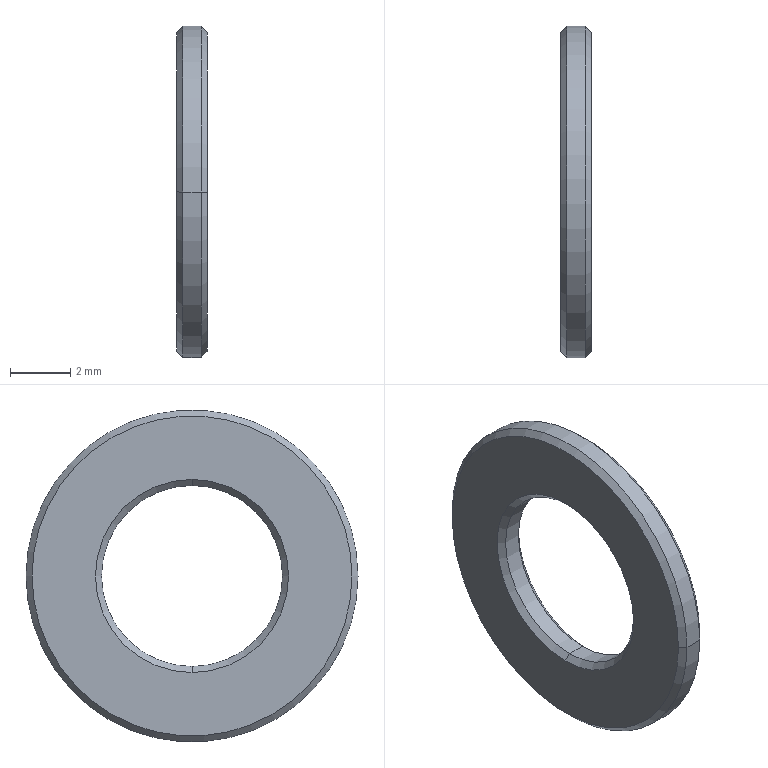Part | STEP file | FWSSS-D11-V6-T1 | 1 solid | 14 faces | box 1 x 11 x 11 mm | volume 64.623 mm3 | cone 8 | cylinder 4 | plane 2 | commonest cylinder face diameters 6 x2 11 x2
STEP:
#1=CARTESIAN_POINT('',(0.,0.,0.));
#2=DIRECTION('',(0.,0.,1.));
#3=DIRECTION('',(1.,0.,0.));
#4=AXIS2_PLACEMENT_3D('',#1,#2,#3);
#5=CARTESIAN_POINT('',(0.2,0.,3.));
#6=VERTEX_POINT('',#5);
#7=CARTESIAN_POINT('',(0.,0.,3.2));
#8=VERTEX_POINT('',#7);
#9=CARTESIAN_POINT('',(0.2,0.,3.));
#10=DIRECTION('',(-0.7071,0.,0.7071));
#11=VECTOR('',#10,1.);
#12=LINE('',#9,#11);
#13=CARTESIAN_POINT('',(0.2,0.,0.));
#14=DIRECTION('',(-1.,0.,0.));
#15=DIRECTION('',(0.,0.,1.));
#16=AXIS2_PLACEMENT_3D('',#13,#14,#15);
#17=CONICAL_SURFACE('',#16,3.,0.7854);
#18=CARTESIAN_POINT('',(6.283,0.));
#19=DIRECTION('',(0.,1.));
#20=VECTOR('',#19,1.);
#21=LINE('',#18,#20);
#22=(GEOMETRIC_REPRESENTATION_CONTEXT(2)PARAMETRIC_REPRESENTATION_CONTEXT()REPRESENTATION_CONTEXT('',''));
#23=DEFINITIONAL_REPRESENTATION('',(#21),#22);
#24=PCURVE('',#17,#23);
#25=CARTESIAN_POINT('',(0.2,0.,0.));
#26=DIRECTION('',(-1.,0.,0.));
#27=DIRECTION('',(0.,0.,1.));
#28=AXIS2_PLACEMENT_3D('',#25,#26,#27);
#29=CONICAL_SURFACE('',#28,3.,0.7854);
#30=CARTESIAN_POINT('',(0.,0.));
#31=DIRECTION('',(0.,1.));
#32=VECTOR('',#31,1.);
#33=LINE('',#30,#32);
#34=(GEOMETRIC_REPRESENTATION_CONTEXT(2)PARAMETRIC_REPRESENTATION_CONTEXT()REPRESENTATION_CONTEXT('',''));
#35=DEFINITIONAL_REPRESENTATION('',(#33),#34);
#36=PCURVE('',#29,#35);
#37=SURFACE_CURVE('',#12,(#24,#36),.PCURVE_S1.);
#38=EDGE_CURVE('',#6,#8,#37,.T.);
#39=ORIENTED_EDGE('',*,*,#38,.T.);
#40=CARTESIAN_POINT('',(0.,0.,-3.2));
#41=VERTEX_POINT('',#40);
#42=CARTESIAN_POINT('',(0.,0.,0.));
#43=DIRECTION('',(1.,0.,0.));
#44=DIRECTION('',(0.,1.,0.));
#45=AXIS2_PLACEMENT_3D('',#42,#43,#44);
#46=CIRCLE('',#45,3.2);
#47=CARTESIAN_POINT('',(7.854,0.2));
#48=DIRECTION('',(-1.,0.));
#49=VECTOR('',#48,1.);
#50=LINE('',#47,#49);
#51=(GEOMETRIC_REPRESENTATION_CONTEXT(2)PARAMETRIC_REPRESENTATION_CONTEXT()REPRESENTATION_CONTEXT('',''));
#52=DEFINITIONAL_REPRESENTATION('',(#50),#51);
#53=PCURVE('',#17,#52);
#54=CARTESIAN_POINT('',(0.,5.5,0.));
#55=DIRECTION('',(1.,0.,0.));
#56=DIRECTION('',(0.,1.,0.));
#57=AXIS2_PLACEMENT_3D('',#54,#55,#56);
#58=PLANE('',#57);
#59=CARTESIAN_POINT('',(-5.5,0.));
#60=DIRECTION('',(1.,0.));
#61=AXIS2_PLACEMENT_2D('',#59,#60);
#62=CIRCLE('',#61,3.2);
#63=(GEOMETRIC_REPRESENTATION_CONTEXT(2)PARAMETRIC_REPRESENTATION_CONTEXT()REPRESENTATION_CONTEXT('',''));
#64=DEFINITIONAL_REPRESENTATION('',(#62),#63);
#65=PCURVE('',#58,#64);
#66=SURFACE_CURVE('',#46,(#53,#65),.PCURVE_S1.);
#67=EDGE_CURVE('',#8,#41,#66,.T.);
#68=ORIENTED_EDGE('',*,*,#67,.T.);
#69=CARTESIAN_POINT('',(0.2,0.,-3.));
#70=VERTEX_POINT('',#69);
#71=CARTESIAN_POINT('',(0.2,0.,-3.));
#72=DIRECTION('',(-0.7071,0.,-0.7071));
#73=VECTOR('',#72,1.);
#74=LINE('',#71,#73);
#75=CARTESIAN_POINT('',(3.142,0.));
#76=DIRECTION('',(0.,1.));
#77=VECTOR('',#76,1.);
#78=LINE('',#75,#77);
#79=(GEOMETRIC_REPRESENTATION_CONTEXT(2)PARAMETRIC_REPRESENTATION_CONTEXT()REPRESENTATION_CONTEXT('',''));
#80=DEFINITIONAL_REPRESENTATION('',(#78),#79);
#81=PCURVE('',#17,#80);
#82=CARTESIAN_POINT('',(3.142,0.));
#83=DIRECTION('',(0.,1.));
#84=VECTOR('',#83,1.);
#85=LINE('',#82,#84);
#86=(GEOMETRIC_REPRESENTATION_CONTEXT(2)PARAMETRIC_REPRESENTATION_CONTEXT()REPRESENTATION_CONTEXT('',''));
#87=DEFINITIONAL_REPRESENTATION('',(#85),#86);
#88=PCURVE('',#29,#87);
#89=SURFACE_CURVE('',#74,(#81,#88),.PCURVE_S1.);
#90=EDGE_CURVE('',#70,#41,#89,.T.);
#91=ORIENTED_EDGE('',*,*,#90,.F.);
#92=CARTESIAN_POINT('',(0.2,0.,0.));
#93=DIRECTION('',(-1.,0.,0.));
#94=DIRECTION('',(0.,0.,-1.));
#95=AXIS2_PLACEMENT_3D('',#92,#93,#94);
#96=CIRCLE('',#95,3.);
#97=CARTESIAN_POINT('',(3.142,0.));
#98=DIRECTION('',(1.,0.));
#99=VECTOR('',#98,1.);
#100=LINE('',#97,#99);
#101=(GEOMETRIC_REPRESENTATION_CONTEXT(2)PARAMETRIC_REPRESENTATION_CONTEXT()REPRESENTATION_CONTEXT('',''));
#102=DEFINITIONAL_REPRESENTATION('',(#100),#101);
#103=PCURVE('',#17,#102);
#104=CARTESIAN_POINT('',(0.,0.,0.));
#105=DIRECTION('',(1.,0.,0.));
#106=DIRECTION('',(0.,0.,-1.));
#107=AXIS2_PLACEMENT_3D('',#104,#105,#106);
#108=CYLINDRICAL_SURFACE('',#107,3.);
#109=CARTESIAN_POINT('',(6.283,0.2));
#110=DIRECTION('',(-1.,0.));
#111=VECTOR('',#110,1.);
#112=LINE('',#109,#111);
#113=(GEOMETRIC_REPRESENTATION_CONTEXT(2)PARAMETRIC_REPRESENTATION_CONTEXT()REPRESENTATION_CONTEXT('',''));
#114=DEFINITIONAL_REPRESENTATION('',(#112),#113);
#115=PCURVE('',#108,#114);
#116=SURFACE_CURVE('',#96,(#103,#115),.PCURVE_S1.);
#117=EDGE_CURVE('',#70,#6,#116,.T.);
#118=ORIENTED_EDGE('',*,*,#117,.T.);
#119=EDGE_LOOP('',(#39,#68,#91,#118));
#120=FACE_BOUND('',#119,.F.);
#121=ADVANCED_FACE('',(#120),#17,.F.);
#122=CARTESIAN_POINT('',(0.8,0.,-3.));
#123=VERTEX_POINT('',#122);
#124=CARTESIAN_POINT('',(1.,0.,-3.2));
#125=VERTEX_POINT('',#124);
#126=CARTESIAN_POINT('',(0.8,0.,-3.));
#127=DIRECTION('',(0.7071,0.,-0.7071));
#128=VECTOR('',#127,1.);
#129=LINE('',#126,#128);
#130=CARTESIAN_POINT('',(0.8,0.,0.));
#131=DIRECTION('',(1.,0.,0.));
#132=DIRECTION('',(0.,0.,-1.));
#133=AXIS2_PLACEMENT_3D('',#130,#131,#132);
#134=CONICAL_SURFACE('',#133,3.,0.7854);
#135=CARTESIAN_POINT('',(6.283,0.));
#136=DIRECTION('',(0.,1.));
#137=VECTOR('',#136,1.);
#138=LINE('',#135,#137);
#139=(GEOMETRIC_REPRESENTATION_CONTEXT(2)PARAMETRIC_REPRESENTATION_CONTEXT()REPRESENTATION_CONTEXT('',''));
#140=DEFINITIONAL_REPRESENTATION('',(#138),#139);
#141=PCURVE('',#134,#140);
#142=CARTESIAN_POINT('',(0.8,0.,0.));
#143=DIRECTION('',(1.,0.,0.));
#144=DIRECTION('',(0.,0.,-1.));
#145=AXIS2_PLACEMENT_3D('',#142,#143,#144);
#146=CONICAL_SURFACE('',#145,3.,0.7854);
#147=CARTESIAN_POINT('',(0.,0.));
#148=DIRECTION('',(0.,1.));
#149=VECTOR('',#148,1.);
#150=LINE('',#147,#149);
#151=(GEOMETRIC_REPRESENTATION_CONTEXT(2)PARAMETRIC_REPRESENTATION_CONTEXT()REPRESENTATION_CONTEXT('',''));
#152=DEFINITIONAL_REPRESENTATION('',(#150),#151);
#153=PCURVE('',#146,#152);
#154=SURFACE_CURVE('',#129,(#141,#153),.PCURVE_S1.);
#155=EDGE_CURVE('',#123,#125,#154,.T.);
#156=ORIENTED_EDGE('',*,*,#155,.T.);
#157=CARTESIAN_POINT('',(1.,0.,3.2));
#158=VERTEX_POINT('',#157);
#159=CARTESIAN_POINT('',(1.,0.,0.));
#160=DIRECTION('',(-1.,0.,0.));
#161=DIRECTION('',(0.,-1.,0.));
#162=AXIS2_PLACEMENT_3D('',#159,#160,#161);
#163=CIRCLE('',#162,3.2);
#164=CARTESIAN_POINT('',(10.996,0.2));
#165=DIRECTION('',(-1.,0.));
#166=VECTOR('',#165,1.);
#167=LINE('',#164,#166);
#168=(GEOMETRIC_REPRESENTATION_CONTEXT(2)PARAMETRIC_REPRESENTATION_CONTEXT()REPRESENTATION_CONTEXT('',''));
#169=DEFINITIONAL_REPRESENTATION('',(#167),#168);
#170=PCURVE('',#134,#169);
#171=CARTESIAN_POINT('',(1.,5.5,0.));
#172=DIRECTION('',(-1.,0.,0.));
#173=DIRECTION('',(0.,-1.,0.));
#174=AXIS2_PLACEMENT_3D('',#171,#172,#173);
#175=PLANE('',#174);
#176=CARTESIAN_POINT('',(5.5,0.));
#177=DIRECTION('',(1.,0.));
#178=AXIS2_PLACEMENT_2D('',#176,#177);
#179=CIRCLE('',#178,3.2);
#180=(GEOMETRIC_REPRESENTATION_CONTEXT(2)PARAMETRIC_REPRESENTATION_CONTEXT()REPRESENTATION_CONTEXT('',''));
#181=DEFINITIONAL_REPRESENTATION('',(#179),#180);
#182=PCURVE('',#175,#181);
#183=SURFACE_CURVE('',#163,(#170,#182),.PCURVE_S1.);
#184=EDGE_CURVE('',#125,#158,#183,.T.);
#185=ORIENTED_EDGE('',*,*,#184,.T.);
#186=CARTESIAN_POINT('',(0.8,0.,3.));
#187=VERTEX_POINT('',#186);
#188=CARTESIAN_POINT('',(0.8,0.,3.));
#189=DIRECTION('',(0.7071,0.,0.7071));
#190=VECTOR('',#189,1.);
#191=LINE('',#188,#190);
#192=CARTESIAN_POINT('',(3.142,0.));
#193=DIRECTION('',(0.,1.));
#194=VECTOR('',#193,1.);
#195=LINE('',#192,#194);
#196=(GEOMETRIC_REPRESENTATION_CONTEXT(2)PARAMETRIC_REPRESENTATION_CONTEXT()REPRESENTATION_CONTEXT('',''));
#197=DEFINITIONAL_REPRESENTATION('',(#195),#196);
#198=PCURVE('',#134,#197);
#199=CARTESIAN_POINT('',(3.142,0.));
#200=DIRECTION('',(0.,1.));
#201=VECTOR('',#200,1.);
#202=LINE('',#199,#201);
#203=(GEOMETRIC_REPRESENTATION_CONTEXT(2)PARAMETRIC_REPRESENTATION_CONTEXT()REPRESENTATION_CONTEXT('',''));
#204=DEFINITIONAL_REPRESENTATION('',(#202),#203);
#205=PCURVE('',#146,#204);
#206=SURFACE_CURVE('',#191,(#198,#205),.PCURVE_S1.);
#207=EDGE_CURVE('',#187,#158,#206,.T.);
#208=ORIENTED_EDGE('',*,*,#207,.F.);
#209=CARTESIAN_POINT('',(0.8,0.,0.));
#210=DIRECTION('',(1.,0.,0.));
#211=DIRECTION('',(0.,0.,1.));
#212=AXIS2_PLACEMENT_3D('',#209,#210,#211);
#213=CIRCLE('',#212,3.);
#214=CARTESIAN_POINT('',(3.142,0.));
#215=DIRECTION('',(1.,0.));
#216=VECTOR('',#215,1.);
#217=LINE('',#214,#216);
#218=(GEOMETRIC_REPRESENTATION_CONTEXT(2)PARAMETRIC_REPRESENTATION_CONTEXT()REPRESENTATION_CONTEXT('',''));
#219=DEFINITIONAL_REPRESENTATION('',(#217),#218);
#220=PCURVE('',#134,#219);
#221=CARTESIAN_POINT('',(3.142,0.8));
#222=DIRECTION('',(1.,0.));
#223=VECTOR('',#222,1.);
#224=LINE('',#221,#223);
#225=(GEOMETRIC_REPRESENTATION_CONTEXT(2)PARAMETRIC_REPRESENTATION_CONTEXT()REPRESENTATION_CONTEXT('',''));
#226=DEFINITIONAL_REPRESENTATION('',(#224),#225);
#227=PCURVE('',#108,#226);
#228=SURFACE_CURVE('',#213,(#220,#227),.PCURVE_S1.);
#229=EDGE_CURVE('',#187,#123,#228,.T.);
#230=ORIENTED_EDGE('',*,*,#229,.T.);
#231=EDGE_LOOP('',(#156,#185,#208,#230));
#232=FACE_BOUND('',#231,.F.);
#233=ADVANCED_FACE('',(#232),#134,.F.);
#234=CARTESIAN_POINT('',(1.,5.3,0.));
#235=VERTEX_POINT('',#234);
#236=CARTESIAN_POINT('',(1.,-5.3,0.));
#237=VERTEX_POINT('',#236);
#238=CARTESIAN_POINT('',(1.,0.,0.));
#239=DIRECTION('',(1.,0.,0.));
#240=DIRECTION('',(0.,-1.,0.));
#241=AXIS2_PLACEMENT_3D('',#238,#239,#240);
#242=CIRCLE('',#241,5.3);
#243=CARTESIAN_POINT('',(0.8,0.,0.));
#244=DIRECTION('',(-1.,0.,0.));
#245=DIRECTION('',(0.,-1.,0.));
#246=AXIS2_PLACEMENT_3D('',#243,#244,#245);
#247=CONICAL_SURFACE('',#246,5.5,0.7854);
#248=CARTESIAN_POINT('',(6.283,-0.2));
#249=DIRECTION('',(-1.,0.));
#250=VECTOR('',#249,1.);
#251=LINE('',#248,#250);
#252=(GEOMETRIC_REPRESENTATION_CONTEXT(2)PARAMETRIC_REPRESENTATION_CONTEXT()REPRESENTATION_CONTEXT('',''));
#253=DEFINITIONAL_REPRESENTATION('',(#251),#252);
#254=PCURVE('',#247,#253);
#255=CARTESIAN_POINT('',(10.8,0.));
#256=CARTESIAN_POINT('',(10.8,-9.18));
#257=CARTESIAN_POINT('',(2.85,-4.59));
#258=CARTESIAN_POINT('',(-5.1,0.));
#259=CARTESIAN_POINT('',(2.85,4.59));
#260=CARTESIAN_POINT('',(10.8,9.18));
#261=CARTESIAN_POINT('',(10.8,0.));
#262=(BOUNDED_CURVE()B_SPLINE_CURVE(2,(#255,#256,#257,#258,#259,#260,#261),.UNSPECIFIED.,.T.,.F.)B_SPLINE_CURVE_WITH_KNOTS((1,2,2,2,2,1),(-2.094,0.,2.094,4.189,6.283,8.378),.UNSPECIFIED.)CURVE()GEOMETRIC_REPRESENTATION_ITEM()RATIONAL_B_SPLINE_CURVE((1.,0.5,1.,0.5,1.,0.5,1.))REPRESENTATION_ITEM(''));
#263=(GEOMETRIC_REPRESENTATION_CONTEXT(2)PARAMETRIC_REPRESENTATION_CONTEXT()REPRESENTATION_CONTEXT('',''));
#264=DEFINITIONAL_REPRESENTATION('',(#262),#263);
#265=PCURVE('',#175,#264);
#266=SURFACE_CURVE('',#242,(#254,#265),.PCURVE_S1.);
#267=EDGE_CURVE('',#235,#237,#266,.T.);
#268=ORIENTED_EDGE('',*,*,#267,.F.);
#269=CARTESIAN_POINT('',(0.8,5.5,0.));
#270=VERTEX_POINT('',#269);
#271=CARTESIAN_POINT('',(0.8,5.5,0.));
#272=DIRECTION('',(-0.7071,0.7071,0.));
#273=VECTOR('',#272,1.);
#274=LINE('',#271,#273);
#275=CARTESIAN_POINT('',(3.142,0.));
#276=DIRECTION('',(0.,1.));
#277=VECTOR('',#276,1.);
#278=LINE('',#275,#277);
#279=(GEOMETRIC_REPRESENTATION_CONTEXT(2)PARAMETRIC_REPRESENTATION_CONTEXT()REPRESENTATION_CONTEXT('',''));
#280=DEFINITIONAL_REPRESENTATION('',(#278),#279);
#281=PCURVE('',#247,#280);
#282=CARTESIAN_POINT('',(0.8,0.,0.));
#283=DIRECTION('',(-1.,0.,0.));
#284=DIRECTION('',(0.,-1.,0.));
#285=AXIS2_PLACEMENT_3D('',#282,#283,#284);
#286=CONICAL_SURFACE('',#285,5.5,0.7854);
#287=CARTESIAN_POINT('',(3.142,0.));
#288=DIRECTION('',(0.,1.));
#289=VECTOR('',#288,1.);
#290=LINE('',#287,#289);
#291=(GEOMETRIC_REPRESENTATION_CONTEXT(2)PARAMETRIC_REPRESENTATION_CONTEXT()REPRESENTATION_CONTEXT('',''));
#292=DEFINITIONAL_REPRESENTATION('',(#290),#291);
#293=PCURVE('',#286,#292);
#294=SURFACE_CURVE('',#274,(#281,#293),.PCURVE_S1.);
#295=EDGE_CURVE('',#235,#270,#294,.T.);
#296=ORIENTED_EDGE('',*,*,#295,.T.);
#297=CARTESIAN_POINT('',(0.8,-5.5,0.));
#298=VERTEX_POINT('',#297);
#299=CARTESIAN_POINT('',(0.8,0.,0.));
#300=DIRECTION('',(-1.,0.,0.));
#301=DIRECTION('',(0.,-1.,0.));
#302=AXIS2_PLACEMENT_3D('',#299,#300,#301);
#303=CIRCLE('',#302,5.5);
#304=CARTESIAN_POINT('',(0.,0.));
#305=DIRECTION('',(1.,0.));
#306=VECTOR('',#305,1.);
#307=LINE('',#304,#306);
#308=(GEOMETRIC_REPRESENTATION_CONTEXT(2)PARAMETRIC_REPRESENTATION_CONTEXT()REPRESENTATION_CONTEXT('',''));
#309=DEFINITIONAL_REPRESENTATION('',(#307),#308);
#310=PCURVE('',#247,#309);
#311=CARTESIAN_POINT('',(0.,0.,0.));
#312=DIRECTION('',(-1.,0.,0.));
#313=DIRECTION('',(0.,-1.,0.));
#314=AXIS2_PLACEMENT_3D('',#311,#312,#313);
#315=CYLINDRICAL_SURFACE('',#314,5.5);
#316=CARTESIAN_POINT('',(0.,-0.8));
#317=DIRECTION('',(1.,0.));
#318=VECTOR('',#317,1.);
#319=LINE('',#316,#318);
#320=(GEOMETRIC_REPRESENTATION_CONTEXT(2)PARAMETRIC_REPRESENTATION_CONTEXT()REPRESENTATION_CONTEXT('',''));
#321=DEFINITIONAL_REPRESENTATION('',(#319),#320);
#322=PCURVE('',#315,#321);
#323=SURFACE_CURVE('',#303,(#310,#322),.PCURVE_S1.);
#324=EDGE_CURVE('',#298,#270,#323,.T.);
#325=ORIENTED_EDGE('',*,*,#324,.F.);
#326=CARTESIAN_POINT('',(0.8,-5.5,0.));
#327=DIRECTION('',(-0.7071,-0.7071,0.));
#328=VECTOR('',#327,1.);
#329=LINE('',#326,#328);
#330=CARTESIAN_POINT('',(0.,0.));
#331=DIRECTION('',(0.,1.));
#332=VECTOR('',#331,1.);
#333=LINE('',#330,#332);
#334=(GEOMETRIC_REPRESENTATION_CONTEXT(2)PARAMETRIC_REPRESENTATION_CONTEXT()REPRESENTATION_CONTEXT('',''));
#335=DEFINITIONAL_REPRESENTATION('',(#333),#334);
#336=PCURVE('',#247,#335);
#337=CARTESIAN_POINT('',(6.283,0.));
#338=DIRECTION('',(0.,1.));
#339=VECTOR('',#338,1.);
#340=LINE('',#337,#339);
#341=(GEOMETRIC_REPRESENTATION_CONTEXT(2)PARAMETRIC_REPRESENTATION_CONTEXT()REPRESENTATION_CONTEXT('',''));
#342=DEFINITIONAL_REPRESENTATION('',(#340),#341);
#343=PCURVE('',#286,#342);
#344=SURFACE_CURVE('',#329,(#336,#343),.PCURVE_S1.);
#345=EDGE_CURVE('',#237,#298,#344,.T.);
#346=ORIENTED_EDGE('',*,*,#345,.F.);
#347=EDGE_LOOP('',(#268,#296,#325,#346));
#348=FACE_BOUND('',#347,.T.);
#349=ADVANCED_FACE('',(#348),#247,.T.);
#350=CARTESIAN_POINT('',(0.,-5.3,0.));
#351=VERTEX_POINT('',#350);
#352=CARTESIAN_POINT('',(0.,5.3,0.));
#353=VERTEX_POINT('',#352);
#354=CARTESIAN_POINT('',(0.,0.,0.));
#355=DIRECTION('',(-1.,0.,0.));
#356=DIRECTION('',(0.,1.,0.));
#357=AXIS2_PLACEMENT_3D('',#354,#355,#356);
#358=CIRCLE('',#357,5.3);
#359=CARTESIAN_POINT('',(0.,0.,0.));
#360=DIRECTION('',(1.,0.,0.));
#361=DIRECTION('',(0.,1.,0.));
#362=AXIS2_PLACEMENT_3D('',#359,#360,#361);
#363=CONICAL_SURFACE('',#362,5.3,0.7854);
#364=CARTESIAN_POINT('',(6.283,0.));
#365=DIRECTION('',(-1.,0.));
#366=VECTOR('',#365,1.);
#367=LINE('',#364,#366);
#368=(GEOMETRIC_REPRESENTATION_CONTEXT(2)PARAMETRIC_REPRESENTATION_CONTEXT()REPRESENTATION_CONTEXT('',''));
#369=DEFINITIONAL_REPRESENTATION('',(#367),#368);
#370=PCURVE('',#363,#369);
#371=CARTESIAN_POINT('',(-0.2,0.));
#372=CARTESIAN_POINT('',(-0.2,-9.18));
#373=CARTESIAN_POINT('',(-8.15,-4.59));
#374=CARTESIAN_POINT('',(-16.1,0.));
#375=CARTESIAN_POINT('',(-8.15,4.59));
#376=CARTESIAN_POINT('',(-0.2,9.18));
#377=CARTESIAN_POINT('',(-0.2,0.));
#378=(BOUNDED_CURVE()B_SPLINE_CURVE(2,(#371,#372,#373,#374,#375,#376,#377),.UNSPECIFIED.,.T.,.F.)B_SPLINE_CURVE_WITH_KNOTS((1,2,2,2,2,1),(-2.094,0.,2.094,4.189,6.283,8.378),.UNSPECIFIED.)CURVE()GEOMETRIC_REPRESENTATION_ITEM()RATIONAL_B_SPLINE_CURVE((1.,0.5,1.,0.5,1.,0.5,1.))REPRESENTATION_ITEM(''));
#379=(GEOMETRIC_REPRESENTATION_CONTEXT(2)PARAMETRIC_REPRESENTATION_CONTEXT()REPRESENTATION_CONTEXT('',''));
#380=DEFINITIONAL_REPRESENTATION('',(#378),#379);
#381=PCURVE('',#58,#380);
#382=SURFACE_CURVE('',#358,(#370,#381),.PCURVE_S1.);
#383=EDGE_CURVE('',#351,#353,#382,.T.);
#384=ORIENTED_EDGE('',*,*,#383,.F.);
#385=CARTESIAN_POINT('',(0.2,-5.5,0.));
#386=VERTEX_POINT('',#385);
#387=CARTESIAN_POINT('',(0.,-5.3,0.));
#388=DIRECTION('',(0.7071,-0.7071,0.));
#389=VECTOR('',#388,1.);
#390=LINE('',#387,#389);
#391=CARTESIAN_POINT('',(3.142,0.));
#392=DIRECTION('',(0.,1.));
#393=VECTOR('',#392,1.);
#394=LINE('',#391,#393);
#395=(GEOMETRIC_REPRESENTATION_CONTEXT(2)PARAMETRIC_REPRESENTATION_CONTEXT()REPRESENTATION_CONTEXT('',''));
#396=DEFINITIONAL_REPRESENTATION('',(#394),#395);
#397=PCURVE('',#363,#396);
#398=CARTESIAN_POINT('',(0.,0.,0.));
#399=DIRECTION('',(1.,0.,0.));
#400=DIRECTION('',(0.,1.,0.));
#401=AXIS2_PLACEMENT_3D('',#398,#399,#400);
#402=CONICAL_SURFACE('',#401,5.3,0.7854);
#403=CARTESIAN_POINT('',(3.142,0.));
#404=DIRECTION('',(0.,1.));
#405=VECTOR('',#404,1.);
#406=LINE('',#403,#405);
#407=(GEOMETRIC_REPRESENTATION_CONTEXT(2)PARAMETRIC_REPRESENTATION_CONTEXT()REPRESENTATION_CONTEXT('',''));
#408=DEFINITIONAL_REPRESENTATION('',(#406),#407);
#409=PCURVE('',#402,#408);
#410=SURFACE_CURVE('',#390,(#397,#409),.PCURVE_S1.);
#411=EDGE_CURVE('',#351,#386,#410,.T.);
#412=ORIENTED_EDGE('',*,*,#411,.T.);
#413=CARTESIAN_POINT('',(0.2,5.5,0.));
#414=VERTEX_POINT('',#413);
#415=CARTESIAN_POINT('',(0.2,0.,0.));
#416=DIRECTION('',(1.,0.,0.));
#417=DIRECTION('',(0.,1.,0.));
#418=AXIS2_PLACEMENT_3D('',#415,#416,#417);
#419=CIRCLE('',#418,5.5);
#420=CARTESIAN_POINT('',(0.,0.2));
#421=DIRECTION('',(1.,0.));
#422=VECTOR('',#421,1.);
#423=LINE('',#420,#422);
#424=(GEOMETRIC_REPRESENTATION_CONTEXT(2)PARAMETRIC_REPRESENTATION_CONTEXT()REPRESENTATION_CONTEXT('',''));
#425=DEFINITIONAL_REPRESENTATION('',(#423),#424);
#426=PCURVE('',#363,#425);
#427=CARTESIAN_POINT('',(3.142,-0.2));
#428=DIRECTION('',(-1.,0.));
#429=VECTOR('',#428,1.);
#430=LINE('',#427,#429);
#431=(GEOMETRIC_REPRESENTATION_CONTEXT(2)PARAMETRIC_REPRESENTATION_CONTEXT()REPRESENTATION_CONTEXT('',''));
#432=DEFINITIONAL_REPRESENTATION('',(#430),#431);
#433=PCURVE('',#315,#432);
#434=SURFACE_CURVE('',#419,(#426,#433),.PCURVE_S1.);
#435=EDGE_CURVE('',#414,#386,#434,.T.);
#436=ORIENTED_EDGE('',*,*,#435,.F.);
#437=CARTESIAN_POINT('',(0.,5.3,0.));
#438=DIRECTION('',(0.7071,0.7071,0.));
#439=VECTOR('',#438,1.);
#440=LINE('',#437,#439);
#441=CARTESIAN_POINT('',(0.,0.));
#442=DIRECTION('',(0.,1.));
#443=VECTOR('',#442,1.);
#444=LINE('',#441,#443);
#445=(GEOMETRIC_REPRESENTATION_CONTEXT(2)PARAMETRIC_REPRESENTATION_CONTEXT()REPRESENTATION_CONTEXT('',''));
#446=DEFINITIONAL_REPRESENTATION('',(#444),#445);
#447=PCURVE('',#363,#446);
#448=CARTESIAN_POINT('',(6.283,0.));
#449=DIRECTION('',(0.,1.));
#450=VECTOR('',#449,1.);
#451=LINE('',#448,#450);
#452=(GEOMETRIC_REPRESENTATION_CONTEXT(2)PARAMETRIC_REPRESENTATION_CONTEXT()REPRESENTATION_CONTEXT('',''));
#453=DEFINITIONAL_REPRESENTATION('',(#451),#452);
#454=PCURVE('',#402,#453);
#455=SURFACE_CURVE('',#440,(#447,#454),.PCURVE_S1.);
#456=EDGE_CURVE('',#353,#414,#455,.T.);
#457=ORIENTED_EDGE('',*,*,#456,.F.);
#458=EDGE_LOOP('',(#384,#412,#436,#457));
#459=FACE_BOUND('',#458,.T.);
#460=ADVANCED_FACE('',(#459),#363,.T.);
#461=CARTESIAN_POINT('',(0.,0.,-3.));
#462=DIRECTION('',(1.,0.,0.));
#463=VECTOR('',#462,1.);
#464=LINE('',#461,#463);
#465=CARTESIAN_POINT('',(6.283,0.));
#466=DIRECTION('',(0.,1.));
#467=VECTOR('',#466,1.);
#468=LINE('',#465,#467);
#469=(GEOMETRIC_REPRESENTATION_CONTEXT(2)PARAMETRIC_REPRESENTATION_CONTEXT()REPRESENTATION_CONTEXT('',''));
#470=DEFINITIONAL_REPRESENTATION('',(#468),#469);
#471=PCURVE('',#108,#470);
#472=CARTESIAN_POINT('',(0.,0.,0.));
#473=DIRECTION('',(1.,0.,0.));
#474=DIRECTION('',(0.,0.,-1.));
#475=AXIS2_PLACEMENT_3D('',#472,#473,#474);
#476=CYLINDRICAL_SURFACE('',#475,3.);
#477=CARTESIAN_POINT('',(0.,0.));
#478=DIRECTION('',(0.,1.));
#479=VECTOR('',#478,1.);
#480=LINE('',#477,#479);
#481=(GEOMETRIC_REPRESENTATION_CONTEXT(2)PARAMETRIC_REPRESENTATION_CONTEXT()REPRESENTATION_CONTEXT('',''));
#482=DEFINITIONAL_REPRESENTATION('',(#480),#481);
#483=PCURVE('',#476,#482);
#484=SURFACE_CURVE('',#464,(#471,#483),.PCURVE_S1.);
#485=EDGE_CURVE('',#70,#123,#484,.T.);
#486=ORIENTED_EDGE('',*,*,#485,.T.);
#487=ORIENTED_EDGE('',*,*,#229,.F.);
#488=CARTESIAN_POINT('',(0.,0.,3.));
#489=DIRECTION('',(1.,0.,0.));
#490=VECTOR('',#489,1.);
#491=LINE('',#488,#490);
#492=CARTESIAN_POINT('',(3.142,0.));
#493=DIRECTION('',(0.,1.));
#494=VECTOR('',#493,1.);
#495=LINE('',#492,#494);
#496=(GEOMETRIC_REPRESENTATION_CONTEXT(2)PARAMETRIC_REPRESENTATION_CONTEXT()REPRESENTATION_CONTEXT('',''));
#497=DEFINITIONAL_REPRESENTATION('',(#495),#496);
#498=PCURVE('',#108,#497);
#499=CARTESIAN_POINT('',(3.142,0.));
#500=DIRECTION('',(0.,1.));
#501=VECTOR('',#500,1.);
#502=LINE('',#499,#501);
#503=(GEOMETRIC_REPRESENTATION_CONTEXT(2)PARAMETRIC_REPRESENTATION_CONTEXT()REPRESENTATION_CONTEXT('',''));
#504=DEFINITIONAL_REPRESENTATION('',(#502),#503);
#505=PCURVE('',#476,#504);
#506=SURFACE_CURVE('',#491,(#498,#505),.PCURVE_S1.);
#507=EDGE_CURVE('',#6,#187,#506,.T.);
#508=ORIENTED_EDGE('',*,*,#507,.F.);
#509=ORIENTED_EDGE('',*,*,#117,.F.);
#510=EDGE_LOOP('',(#486,#487,#508,#509));
#511=FACE_BOUND('',#510,.F.);
#512=ADVANCED_FACE('',(#511),#108,.F.);
#513=ORIENTED_EDGE('',*,*,#324,.T.);
#514=CARTESIAN_POINT('',(0.,5.5,0.));
#515=DIRECTION('',(-1.,0.,0.));
#516=VECTOR('',#515,1.);
#517=LINE('',#514,#516);
#518=CARTESIAN_POINT('',(3.142,0.));
#519=DIRECTION('',(0.,1.));
#520=VECTOR('',#519,1.);
#521=LINE('',#518,#520);
#522=(GEOMETRIC_REPRESENTATION_CONTEXT(2)PARAMETRIC_REPRESENTATION_CONTEXT()REPRESENTATION_CONTEXT('',''));
#523=DEFINITIONAL_REPRESENTATION('',(#521),#522);
#524=PCURVE('',#315,#523);
#525=CARTESIAN_POINT('',(0.,0.,0.));
#526=DIRECTION('',(-1.,0.,0.));
#527=DIRECTION('',(0.,-1.,0.));
#528=AXIS2_PLACEMENT_3D('',#525,#526,#527);
#529=CYLINDRICAL_SURFACE('',#528,5.5);
#530=CARTESIAN_POINT('',(3.142,0.));
#531=DIRECTION('',(0.,1.));
#532=VECTOR('',#531,1.);
#533=LINE('',#530,#532);
#534=(GEOMETRIC_REPRESENTATION_CONTEXT(2)PARAMETRIC_REPRESENTATION_CONTEXT()REPRESENTATION_CONTEXT('',''));
#535=DEFINITIONAL_REPRESENTATION('',(#533),#534);
#536=PCURVE('',#529,#535);
#537=SURFACE_CURVE('',#517,(#524,#536),.PCURVE_S1.);
#538=EDGE_CURVE('',#270,#414,#537,.T.);
#539=ORIENTED_EDGE('',*,*,#538,.T.);
#540=ORIENTED_EDGE('',*,*,#435,.T.);
#541=CARTESIAN_POINT('',(0.,-5.5,0.));
#542=DIRECTION('',(-1.,0.,0.));
#543=VECTOR('',#542,1.);
#544=LINE('',#541,#543);
#545=CARTESIAN_POINT('',(0.,0.));
#546=DIRECTION('',(0.,1.));
#547=VECTOR('',#546,1.);
#548=LINE('',#545,#547);
#549=(GEOMETRIC_REPRESENTATION_CONTEXT(2)PARAMETRIC_REPRESENTATION_CONTEXT()REPRESENTATION_CONTEXT('',''));
#550=DEFINITIONAL_REPRESENTATION('',(#548),#549);
#551=PCURVE('',#315,#550);
#552=CARTESIAN_POINT('',(6.283,0.));
#553=DIRECTION('',(0.,1.));
#554=VECTOR('',#553,1.);
#555=LINE('',#552,#554);
#556=(GEOMETRIC_REPRESENTATION_CONTEXT(2)PARAMETRIC_REPRESENTATION_CONTEXT()REPRESENTATION_CONTEXT('',''));
#557=DEFINITIONAL_REPRESENTATION('',(#555),#556);
#558=PCURVE('',#529,#557);
#559=SURFACE_CURVE('',#544,(#551,#558),.PCURVE_S1.);
#560=EDGE_CURVE('',#298,#386,#559,.T.);
#561=ORIENTED_EDGE('',*,*,#560,.F.);
#562=EDGE_LOOP('',(#513,#539,#540,#561));
#563=FACE_BOUND('',#562,.T.);
#564=ADVANCED_FACE('',(#563),#315,.T.);
#565=ORIENTED_EDGE('',*,*,#184,.T.);
#566=CARTESIAN_POINT('',(1.,0.,0.));
#567=DIRECTION('',(-1.,0.,0.));
#568=DIRECTION('',(0.,-1.,0.));
#569=AXIS2_PLACEMENT_3D('',#566,#567,#568);
#570=CIRCLE('',#569,3.2);
#571=CARTESIAN_POINT('',(5.5,0.));
#572=DIRECTION('',(1.,0.));
#573=AXIS2_PLACEMENT_2D('',#571,#572);
#574=CIRCLE('',#573,3.2);
#575=(GEOMETRIC_REPRESENTATION_CONTEXT(2)PARAMETRIC_REPRESENTATION_CONTEXT()REPRESENTATION_CONTEXT('',''));
#576=DEFINITIONAL_REPRESENTATION('',(#574),#575);
#577=PCURVE('',#175,#576);
#578=CARTESIAN_POINT('',(4.712,0.2));
#579=DIRECTION('',(-1.,0.));
#580=VECTOR('',#579,1.);
#581=LINE('',#578,#580);
#582=(GEOMETRIC_REPRESENTATION_CONTEXT(2)PARAMETRIC_REPRESENTATION_CONTEXT()REPRESENTATION_CONTEXT('',''));
#583=DEFINITIONAL_REPRESENTATION('',(#581),#582);
#584=PCURVE('',#146,#583);
#585=SURFACE_CURVE('',#570,(#577,#584),.PCURVE_S1.);
#586=EDGE_CURVE('',#158,#125,#585,.T.);
#587=ORIENTED_EDGE('',*,*,#586,.T.);
#588=EDGE_LOOP('',(#565,#587));
#589=FACE_BOUND('',#588,.T.);
#590=CARTESIAN_POINT('',(1.,0.,0.));
#591=DIRECTION('',(1.,0.,0.));
#592=DIRECTION('',(0.,-1.,0.));
#593=AXIS2_PLACEMENT_3D('',#590,#591,#592);
#594=CIRCLE('',#593,5.3);
#595=CARTESIAN_POINT('',(10.8,0.));
#596=CARTESIAN_POINT('',(10.8,-9.18));
#597=CARTESIAN_POINT('',(2.85,-4.59));
#598=CARTESIAN_POINT('',(-5.1,0.));
#599=CARTESIAN_POINT('',(2.85,4.59));
#600=CARTESIAN_POINT('',(10.8,9.18));
#601=CARTESIAN_POINT('',(10.8,0.));
#602=(BOUNDED_CURVE()B_SPLINE_CURVE(2,(#595,#596,#597,#598,#599,#600,#601),.UNSPECIFIED.,.T.,.F.)B_SPLINE_CURVE_WITH_KNOTS((1,2,2,2,2,1),(-2.094,0.,2.094,4.189,6.283,8.378),.UNSPECIFIED.)CURVE()GEOMETRIC_REPRESENTATION_ITEM()RATIONAL_B_SPLINE_CURVE((1.,0.5,1.,0.5,1.,0.5,1.))REPRESENTATION_ITEM(''));
#603=(GEOMETRIC_REPRESENTATION_CONTEXT(2)PARAMETRIC_REPRESENTATION_CONTEXT()REPRESENTATION_CONTEXT('',''));
#604=DEFINITIONAL_REPRESENTATION('',(#602),#603);
#605=PCURVE('',#175,#604);
#606=CARTESIAN_POINT('',(6.283,-0.2));
#607=DIRECTION('',(-1.,0.));
#608=VECTOR('',#607,1.);
#609=LINE('',#606,#608);
#610=(GEOMETRIC_REPRESENTATION_CONTEXT(2)PARAMETRIC_REPRESENTATION_CONTEXT()REPRESENTATION_CONTEXT('',''));
#611=DEFINITIONAL_REPRESENTATION('',(#609),#610);
#612=PCURVE('',#286,#611);
#613=SURFACE_CURVE('',#594,(#605,#612),.PCURVE_S1.);
#614=EDGE_CURVE('',#237,#235,#613,.T.);
#615=ORIENTED_EDGE('',*,*,#614,.T.);
#616=ORIENTED_EDGE('',*,*,#267,.T.);
#617=EDGE_LOOP('',(#615,#616));
#618=FACE_BOUND('',#617,.T.);
#619=ADVANCED_FACE('',(#589,#618),#175,.F.);
#620=ORIENTED_EDGE('',*,*,#67,.T.);
#621=CARTESIAN_POINT('',(0.,0.,0.));
#622=DIRECTION('',(1.,0.,0.));
#623=DIRECTION('',(0.,1.,0.));
#624=AXIS2_PLACEMENT_3D('',#621,#622,#623);
#625=CIRCLE('',#624,3.2);
#626=CARTESIAN_POINT('',(-5.5,0.));
#627=DIRECTION('',(1.,0.));
#628=AXIS2_PLACEMENT_2D('',#626,#627);
#629=CIRCLE('',#628,3.2);
#630=(GEOMETRIC_REPRESENTATION_CONTEXT(2)PARAMETRIC_REPRESENTATION_CONTEXT()REPRESENTATION_CONTEXT('',''));
#631=DEFINITIONAL_REPRESENTATION('',(#629),#630);
#632=PCURVE('',#58,#631);
#633=CARTESIAN_POINT('',(7.854,0.2));
#634=DIRECTION('',(-1.,0.));
#635=VECTOR('',#634,1.);
#636=LINE('',#633,#635);
#637=(GEOMETRIC_REPRESENTATION_CONTEXT(2)PARAMETRIC_REPRESENTATION_CONTEXT()REPRESENTATION_CONTEXT('',''));
#638=DEFINITIONAL_REPRESENTATION('',(#636),#637);
#639=PCURVE('',#29,#638);
#640=SURFACE_CURVE('',#625,(#632,#639),.PCURVE_S1.);
#641=EDGE_CURVE('',#41,#8,#640,.T.);
#642=ORIENTED_EDGE('',*,*,#641,.T.);
#643=EDGE_LOOP('',(#620,#642));
#644=FACE_BOUND('',#643,.T.);
#645=CARTESIAN_POINT('',(0.,0.,0.));
#646=DIRECTION('',(-1.,0.,0.));
#647=DIRECTION('',(0.,1.,0.));
#648=AXIS2_PLACEMENT_3D('',#645,#646,#647);
#649=CIRCLE('',#648,5.3);
#650=CARTESIAN_POINT('',(-0.2,0.));
#651=CARTESIAN_POINT('',(-0.2,-9.18));
#652=CARTESIAN_POINT('',(-8.15,-4.59));
#653=CARTESIAN_POINT('',(-16.1,0.));
#654=CARTESIAN_POINT('',(-8.15,4.59));
#655=CARTESIAN_POINT('',(-0.2,9.18));
#656=CARTESIAN_POINT('',(-0.2,0.));
#657=(BOUNDED_CURVE()B_SPLINE_CURVE(2,(#650,#651,#652,#653,#654,#655,#656),.UNSPECIFIED.,.T.,.F.)B_SPLINE_CURVE_WITH_KNOTS((1,2,2,2,2,1),(-2.094,0.,2.094,4.189,6.283,8.378),.UNSPECIFIED.)CURVE()GEOMETRIC_REPRESENTATION_ITEM()RATIONAL_B_SPLINE_CURVE((1.,0.5,1.,0.5,1.,0.5,1.))REPRESENTATION_ITEM(''));
#658=(GEOMETRIC_REPRESENTATION_CONTEXT(2)PARAMETRIC_REPRESENTATION_CONTEXT()REPRESENTATION_CONTEXT('',''));
#659=DEFINITIONAL_REPRESENTATION('',(#657),#658);
#660=PCURVE('',#58,#659);
#661=CARTESIAN_POINT('',(6.283,0.));
#662=DIRECTION('',(-1.,0.));
#663=VECTOR('',#662,1.);
#664=LINE('',#661,#663);
#665=(GEOMETRIC_REPRESENTATION_CONTEXT(2)PARAMETRIC_REPRESENTATION_CONTEXT()REPRESENTATION_CONTEXT('',''));
#666=DEFINITIONAL_REPRESENTATION('',(#664),#665);
#667=PCURVE('',#402,#666);
#668=SURFACE_CURVE('',#649,(#660,#667),.PCURVE_S1.);
#669=EDGE_CURVE('',#353,#351,#668,.T.);
#670=ORIENTED_EDGE('',*,*,#669,.T.);
#671=ORIENTED_EDGE('',*,*,#383,.T.);
#672=EDGE_LOOP('',(#670,#671));
#673=FACE_BOUND('',#672,.T.);
#674=ADVANCED_FACE('',(#644,#673),#58,.F.);
#675=ORIENTED_EDGE('',*,*,#538,.F.);
#676=CARTESIAN_POINT('',(0.8,0.,0.));
#677=DIRECTION('',(-1.,0.,0.));
#678=DIRECTION('',(0.,-1.,0.));
#679=AXIS2_PLACEMENT_3D('',#676,#677,#678);
#680=CIRCLE('',#679,5.5);
#681=CARTESIAN_POINT('',(0.,-0.8));
#682=DIRECTION('',(1.,0.));
#683=VECTOR('',#682,1.);
#684=LINE('',#681,#683);
#685=(GEOMETRIC_REPRESENTATION_CONTEXT(2)PARAMETRIC_REPRESENTATION_CONTEXT()REPRESENTATION_CONTEXT('',''));
#686=DEFINITIONAL_REPRESENTATION('',(#684),#685);
#687=PCURVE('',#529,#686);
#688=CARTESIAN_POINT('',(0.,0.));
#689=DIRECTION('',(1.,0.));
#690=VECTOR('',#689,1.);
#691=LINE('',#688,#690);
#692=(GEOMETRIC_REPRESENTATION_CONTEXT(2)PARAMETRIC_REPRESENTATION_CONTEXT()REPRESENTATION_CONTEXT('',''));
#693=DEFINITIONAL_REPRESENTATION('',(#691),#692);
#694=PCURVE('',#286,#693);
#695=SURFACE_CURVE('',#680,(#687,#694),.PCURVE_S1.);
#696=EDGE_CURVE('',#270,#298,#695,.T.);
#697=ORIENTED_EDGE('',*,*,#696,.T.);
#698=ORIENTED_EDGE('',*,*,#560,.T.);
#699=CARTESIAN_POINT('',(0.2,0.,0.));
#700=DIRECTION('',(1.,0.,0.));
#701=DIRECTION('',(0.,1.,0.));
#702=AXIS2_PLACEMENT_3D('',#699,#700,#701);
#703=CIRCLE('',#702,5.5);
#704=CARTESIAN_POINT('',(9.425,-0.2));
#705=DIRECTION('',(-1.,0.));
#706=VECTOR('',#705,1.);
#707=LINE('',#704,#706);
#708=(GEOMETRIC_REPRESENTATION_CONTEXT(2)PARAMETRIC_REPRESENTATION_CONTEXT()REPRESENTATION_CONTEXT('',''));
#709=DEFINITIONAL_REPRESENTATION('',(#707),#708);
#710=PCURVE('',#529,#709);
#711=CARTESIAN_POINT('',(0.,0.2));
#712=DIRECTION('',(1.,0.));
#713=VECTOR('',#712,1.);
#714=LINE('',#711,#713);
#715=(GEOMETRIC_REPRESENTATION_CONTEXT(2)PARAMETRIC_REPRESENTATION_CONTEXT()REPRESENTATION_CONTEXT('',''));
#716=DEFINITIONAL_REPRESENTATION('',(#714),#715);
#717=PCURVE('',#402,#716);
#718=SURFACE_CURVE('',#703,(#710,#717),.PCURVE_S1.);
#719=EDGE_CURVE('',#386,#414,#718,.T.);
#720=ORIENTED_EDGE('',*,*,#719,.T.);
#721=EDGE_LOOP('',(#675,#697,#698,#720));
#722=FACE_BOUND('',#721,.T.);
#723=ADVANCED_FACE('',(#722),#529,.T.);
#724=CARTESIAN_POINT('',(0.8,0.,0.));
#725=DIRECTION('',(1.,0.,0.));
#726=DIRECTION('',(0.,0.,1.));
#727=AXIS2_PLACEMENT_3D('',#724,#725,#726);
#728=CIRCLE('',#727,3.);
#729=CARTESIAN_POINT('',(-3.142,0.8));
#730=DIRECTION('',(1.,0.));
#731=VECTOR('',#730,1.);
#732=LINE('',#729,#731);
#733=(GEOMETRIC_REPRESENTATION_CONTEXT(2)PARAMETRIC_REPRESENTATION_CONTEXT()REPRESENTATION_CONTEXT('',''));
#734=DEFINITIONAL_REPRESENTATION('',(#732),#733);
#735=PCURVE('',#476,#734);
#736=CARTESIAN_POINT('',(-3.142,0.));
#737=DIRECTION('',(1.,0.));
#738=VECTOR('',#737,1.);
#739=LINE('',#736,#738);
#740=(GEOMETRIC_REPRESENTATION_CONTEXT(2)PARAMETRIC_REPRESENTATION_CONTEXT()REPRESENTATION_CONTEXT('',''));
#741=DEFINITIONAL_REPRESENTATION('',(#739),#740);
#742=PCURVE('',#146,#741);
#743=SURFACE_CURVE('',#728,(#735,#742),.PCURVE_S1.);
#744=EDGE_CURVE('',#123,#187,#743,.T.);
#745=ORIENTED_EDGE('',*,*,#744,.F.);
#746=ORIENTED_EDGE('',*,*,#485,.F.);
#747=CARTESIAN_POINT('',(0.2,0.,0.));
#748=DIRECTION('',(-1.,0.,0.));
#749=DIRECTION('',(0.,0.,-1.));
#750=AXIS2_PLACEMENT_3D('',#747,#748,#749);
#751=CIRCLE('',#750,3.);
#752=CARTESIAN_POINT('',(6.283,0.2));
#753=DIRECTION('',(-1.,0.));
#754=VECTOR('',#753,1.);
#755=LINE('',#752,#754);
#756=(GEOMETRIC_REPRESENTATION_CONTEXT(2)PARAMETRIC_REPRESENTATION_CONTEXT()REPRESENTATION_CONTEXT('',''));
#757=DEFINITIONAL_REPRESENTATION('',(#755),#756);
#758=PCURVE('',#476,#757);
#759=CARTESIAN_POINT('',(-3.142,0.));
#760=DIRECTION('',(1.,0.));
#761=VECTOR('',#760,1.);
#762=LINE('',#759,#761);
#763=(GEOMETRIC_REPRESENTATION_CONTEXT(2)PARAMETRIC_REPRESENTATION_CONTEXT()REPRESENTATION_CONTEXT('',''));
#764=DEFINITIONAL_REPRESENTATION('',(#762),#763);
#765=PCURVE('',#29,#764);
#766=SURFACE_CURVE('',#751,(#758,#765),.PCURVE_S1.);
#767=EDGE_CURVE('',#6,#70,#766,.T.);
#768=ORIENTED_EDGE('',*,*,#767,.F.);
#769=ORIENTED_EDGE('',*,*,#507,.T.);
#770=EDGE_LOOP('',(#745,#746,#768,#769));
#771=FACE_BOUND('',#770,.F.);
#772=ADVANCED_FACE('',(#771),#476,.F.);
#773=ORIENTED_EDGE('',*,*,#411,.F.);
#774=ORIENTED_EDGE('',*,*,#669,.F.);
#775=ORIENTED_EDGE('',*,*,#456,.T.);
#776=ORIENTED_EDGE('',*,*,#719,.F.);
#777=EDGE_LOOP('',(#773,#774,#775,#776));
#778=FACE_BOUND('',#777,.T.);
#779=ADVANCED_FACE('',(#778),#402,.T.);
#780=ORIENTED_EDGE('',*,*,#295,.F.);
#781=ORIENTED_EDGE('',*,*,#614,.F.);
#782=ORIENTED_EDGE('',*,*,#345,.T.);
#783=ORIENTED_EDGE('',*,*,#696,.F.);
#784=EDGE_LOOP('',(#780,#781,#782,#783));
#785=FACE_BOUND('',#784,.T.);
#786=ADVANCED_FACE('',(#785),#286,.T.);
#787=ORIENTED_EDGE('',*,*,#586,.T.);
#788=ORIENTED_EDGE('',*,*,#155,.F.);
#789=ORIENTED_EDGE('',*,*,#744,.T.);
#790=ORIENTED_EDGE('',*,*,#207,.T.);
#791=EDGE_LOOP('',(#787,#788,#789,#790));
#792=FACE_BOUND('',#791,.F.);
#793=ADVANCED_FACE('',(#792),#146,.F.);
#794=ORIENTED_EDGE('',*,*,#641,.T.);
#795=ORIENTED_EDGE('',*,*,#38,.F.);
#796=ORIENTED_EDGE('',*,*,#767,.T.);
#797=ORIENTED_EDGE('',*,*,#90,.T.);
#798=EDGE_LOOP('',(#794,#795,#796,#797));
#799=FACE_BOUND('',#798,.F.);
#800=ADVANCED_FACE('',(#799),#29,.F.);
#801=CLOSED_SHELL('',(#121,#233,#349,#460,#512,#564,#619,#674,#723,#772,#779,#786,#793,#800));
#802=MANIFOLD_SOLID_BREP('',#801);
#803=(LENGTH_UNIT()NAMED_UNIT(*)SI_UNIT(.MILLI.,.METRE.));
#804=UNCERTAINTY_MEASURE_WITH_UNIT(LENGTH_MEASURE(0.0000001),#803,'','');
#805=(NAMED_UNIT(*)PLANE_ANGLE_UNIT()SI_UNIT($,.RADIAN.));
#806=(NAMED_UNIT(*)SI_UNIT($,.STERADIAN.)SOLID_ANGLE_UNIT());
#807=(GEOMETRIC_REPRESENTATION_CONTEXT(3)GLOBAL_UNCERTAINTY_ASSIGNED_CONTEXT((#804))GLOBAL_UNIT_ASSIGNED_CONTEXT((#803,#805,#806))REPRESENTATION_CONTEXT('',''));
#808=ADVANCED_BREP_SHAPE_REPRESENTATION('',(#4,#802),#807);